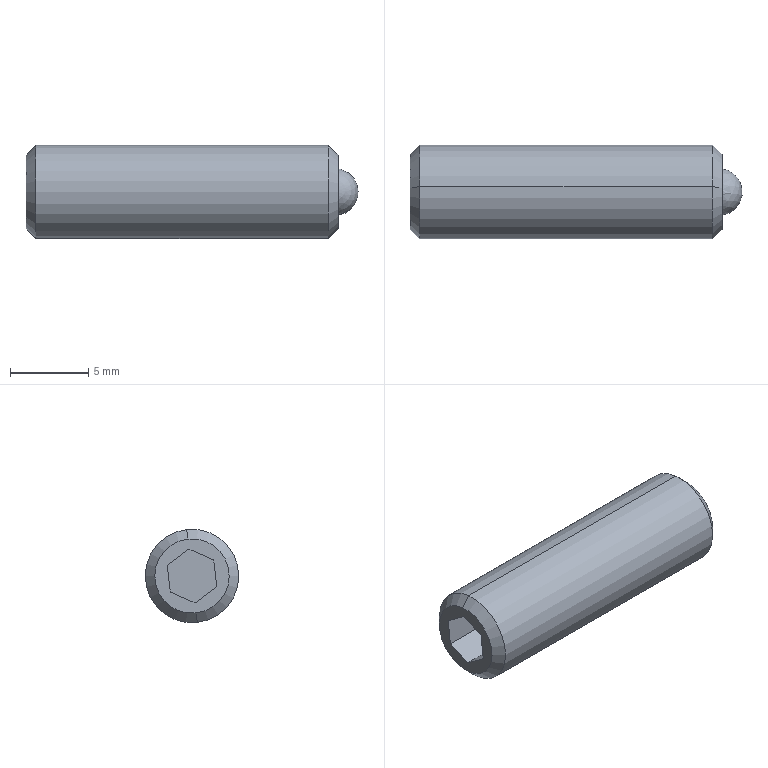Part | NX | features _ZAH01-M6 2 | 1 solid | 16 faces | box 21.3 x 6 x 6 mm | volume 545.053 mm3 | plane 9 | cone 4 | cylinder 2 | sphere 1 | commonest cylinder face diameters 6 x2
STEP:
#1=CARTESIAN_POINT('',(-46.614,117.663,-91.481));
#2=VERTEX_POINT('',#1);
#3=CARTESIAN_POINT('',(-46.614,118.337,-85.519));
#4=VERTEX_POINT('',#3);
#5=CARTESIAN_POINT('',(-46.614,118.,-88.5));
#6=DIRECTION('',(-1.,0.,0.));
#7=DIRECTION('',(0.,-0.1124,-0.9937));
#8=AXIS2_PLACEMENT_3D('',#5,#6,#7);
#9=CIRCLE('',#8,3.);
#10=EDGE_CURVE('',#2,#4,#9,.T.);
#11=ORIENTED_EDGE('',*,*,#10,.T.);
#12=CARTESIAN_POINT('',(-65.386,118.337,-85.519));
#13=VERTEX_POINT('',#12);
#14=CARTESIAN_POINT('',(-46.,118.337,-85.519));
#15=DIRECTION('',(-1.,0.,0.));
#16=VECTOR('',#15,1000.);
#17=LINE('',#14,#16);
#18=EDGE_CURVE('',#4,#13,#17,.T.);
#19=ORIENTED_EDGE('',*,*,#18,.T.);
#20=CARTESIAN_POINT('',(-65.386,117.663,-91.481));
#21=VERTEX_POINT('',#20);
#22=CARTESIAN_POINT('',(-65.386,118.,-88.5));
#23=DIRECTION('',(1.,0.,0.));
#24=DIRECTION('',(0.,-0.1124,-0.9937));
#25=AXIS2_PLACEMENT_3D('',#22,#23,#24);
#26=CIRCLE('',#25,3.);
#27=EDGE_CURVE('',#13,#21,#26,.T.);
#28=ORIENTED_EDGE('',*,*,#27,.T.);
#29=CARTESIAN_POINT('',(-46.,117.663,-91.481));
#30=DIRECTION('',(-1.,0.,0.));
#31=VECTOR('',#30,1000.);
#32=LINE('',#29,#31);
#33=EDGE_CURVE('',#21,#2,#32,.F.);
#34=ORIENTED_EDGE('',*,*,#33,.T.);
#35=EDGE_LOOP('',(#11,#19,#28,#34));
#36=FACE_BOUND('',#35,.T.);
#37=CARTESIAN_POINT('',(-46.,118.,-88.5));
#38=DIRECTION('',(-1.,0.,0.));
#39=DIRECTION('',(0.,0.1124,0.9937));
#40=AXIS2_PLACEMENT_3D('',#37,#38,#39);
#41=CYLINDRICAL_SURFACE('',#40,3.);
#42=ADVANCED_FACE('',(#36),#41,.T.);
#43=CARTESIAN_POINT('',(-66.,118.268,-86.129));
#44=VERTEX_POINT('',#43);
#45=CARTESIAN_POINT('',(-66.,117.732,-90.871));
#46=VERTEX_POINT('',#45);
#47=CARTESIAN_POINT('',(-66.,118.,-88.5));
#48=DIRECTION('',(1.,0.,0.));
#49=DIRECTION('',(0.,0.1124,0.9937));
#50=AXIS2_PLACEMENT_3D('',#47,#48,#49);
#51=CIRCLE('',#50,2.387);
#52=EDGE_CURVE('',#44,#46,#51,.T.);
#53=ORIENTED_EDGE('',*,*,#52,.T.);
#54=CARTESIAN_POINT('',(-65.386,117.663,-91.481));
#55=DIRECTION('',(0.7071,-0.07947,-0.7026));
#56=VECTOR('',#55,1000.);
#57=LINE('',#54,#56);
#58=EDGE_CURVE('',#46,#21,#57,.T.);
#59=ORIENTED_EDGE('',*,*,#58,.T.);
#60=ORIENTED_EDGE('',*,*,#27,.F.);
#61=CARTESIAN_POINT('',(-65.386,118.337,-85.519));
#62=DIRECTION('',(0.7071,0.07947,0.7026));
#63=VECTOR('',#62,1000.);
#64=LINE('',#61,#63);
#65=EDGE_CURVE('',#13,#44,#64,.F.);
#66=ORIENTED_EDGE('',*,*,#65,.T.);
#67=EDGE_LOOP('',(#53,#59,#60,#66));
#68=FACE_BOUND('',#67,.T.);
#69=CARTESIAN_POINT('',(-65.386,118.,-88.5));
#70=DIRECTION('',(1.,0.,0.));
#71=DIRECTION('',(0.,-0.1124,-0.9937));
#72=AXIS2_PLACEMENT_3D('',#69,#70,#71);
#73=CONICAL_SURFACE('',#72,3.,0.7854);
#74=ADVANCED_FACE('',(#68),#73,.T.);
#75=CARTESIAN_POINT('',(-46.,117.732,-90.871));
#76=VERTEX_POINT('',#75);
#77=CARTESIAN_POINT('',(-46.,118.268,-86.129));
#78=VERTEX_POINT('',#77);
#79=CARTESIAN_POINT('',(-46.,118.,-88.5));
#80=DIRECTION('',(-1.,0.,0.));
#81=DIRECTION('',(0.,-0.1124,-0.9937));
#82=AXIS2_PLACEMENT_3D('',#79,#80,#81);
#83=CIRCLE('',#82,2.387);
#84=EDGE_CURVE('',#76,#78,#83,.T.);
#85=ORIENTED_EDGE('',*,*,#84,.T.);
#86=CARTESIAN_POINT('',(-46.614,118.337,-85.519));
#87=DIRECTION('',(-0.7071,0.07947,0.7026));
#88=VECTOR('',#87,1000.);
#89=LINE('',#86,#88);
#90=EDGE_CURVE('',#4,#78,#89,.F.);
#91=ORIENTED_EDGE('',*,*,#90,.F.);
#92=ORIENTED_EDGE('',*,*,#10,.F.);
#93=CARTESIAN_POINT('',(-46.614,117.663,-91.481));
#94=DIRECTION('',(-0.7071,-0.07947,-0.7026));
#95=VECTOR('',#94,1000.);
#96=LINE('',#93,#95);
#97=EDGE_CURVE('',#76,#2,#96,.T.);
#98=ORIENTED_EDGE('',*,*,#97,.F.);
#99=EDGE_LOOP('',(#85,#91,#92,#98));
#100=FACE_BOUND('',#99,.T.);
#101=CARTESIAN_POINT('',(-46.614,118.,-88.5));
#102=DIRECTION('',(-1.,0.,0.));
#103=DIRECTION('',(0.,0.1124,0.9937));
#104=AXIS2_PLACEMENT_3D('',#101,#102,#103);
#105=CONICAL_SURFACE('',#104,3.,0.7854);
#106=ADVANCED_FACE('',(#100),#105,.T.);
#107=ORIENTED_EDGE('',*,*,#18,.F.);
#108=CARTESIAN_POINT('',(-46.614,118.,-88.5));
#109=DIRECTION('',(-1.,0.,0.));
#110=DIRECTION('',(0.,-0.1124,-0.9937));
#111=AXIS2_PLACEMENT_3D('',#108,#109,#110);
#112=CIRCLE('',#111,3.);
#113=EDGE_CURVE('',#4,#2,#112,.T.);
#114=ORIENTED_EDGE('',*,*,#113,.T.);
#115=ORIENTED_EDGE('',*,*,#33,.F.);
#116=CARTESIAN_POINT('',(-65.386,118.,-88.5));
#117=DIRECTION('',(1.,0.,0.));
#118=DIRECTION('',(0.,-0.1124,-0.9937));
#119=AXIS2_PLACEMENT_3D('',#116,#117,#118);
#120=CIRCLE('',#119,3.);
#121=EDGE_CURVE('',#21,#13,#120,.T.);
#122=ORIENTED_EDGE('',*,*,#121,.T.);
#123=EDGE_LOOP('',(#107,#114,#115,#122));
#124=FACE_BOUND('',#123,.T.);
#125=CARTESIAN_POINT('',(-46.,118.,-88.5));
#126=DIRECTION('',(-1.,0.,0.));
#127=DIRECTION('',(0.,0.1124,0.9937));
#128=AXIS2_PLACEMENT_3D('',#125,#126,#127);
#129=CYLINDRICAL_SURFACE('',#128,3.);
#130=ADVANCED_FACE('',(#124),#129,.T.);
#131=ORIENTED_EDGE('',*,*,#58,.F.);
#132=CARTESIAN_POINT('',(-66.,118.,-88.5));
#133=DIRECTION('',(1.,0.,0.));
#134=DIRECTION('',(0.,0.1124,0.9937));
#135=AXIS2_PLACEMENT_3D('',#132,#133,#134);
#136=CIRCLE('',#135,2.387);
#137=EDGE_CURVE('',#46,#44,#136,.T.);
#138=ORIENTED_EDGE('',*,*,#137,.T.);
#139=ORIENTED_EDGE('',*,*,#65,.F.);
#140=ORIENTED_EDGE('',*,*,#121,.F.);
#141=EDGE_LOOP('',(#131,#138,#139,#140));
#142=FACE_BOUND('',#141,.T.);
#143=CARTESIAN_POINT('',(-65.386,118.,-88.5));
#144=DIRECTION('',(1.,0.,0.));
#145=DIRECTION('',(0.,-0.1124,-0.9937));
#146=AXIS2_PLACEMENT_3D('',#143,#144,#145);
#147=CONICAL_SURFACE('',#146,3.,0.7854);
#148=ADVANCED_FACE('',(#142),#147,.T.);
#149=ORIENTED_EDGE('',*,*,#90,.T.);
#150=CARTESIAN_POINT('',(-46.,118.,-88.5));
#151=DIRECTION('',(-1.,0.,0.));
#152=DIRECTION('',(0.,-0.1124,-0.9937));
#153=AXIS2_PLACEMENT_3D('',#150,#151,#152);
#154=CIRCLE('',#153,2.387);
#155=EDGE_CURVE('',#78,#76,#154,.T.);
#156=ORIENTED_EDGE('',*,*,#155,.T.);
#157=ORIENTED_EDGE('',*,*,#97,.T.);
#158=ORIENTED_EDGE('',*,*,#113,.F.);
#159=EDGE_LOOP('',(#149,#156,#157,#158));
#160=FACE_BOUND('',#159,.T.);
#161=CARTESIAN_POINT('',(-46.614,118.,-88.5));
#162=DIRECTION('',(-1.,0.,0.));
#163=DIRECTION('',(0.,0.1124,0.9937));
#164=AXIS2_PLACEMENT_3D('',#161,#162,#163);
#165=CONICAL_SURFACE('',#164,3.,0.7854);
#166=ADVANCED_FACE('',(#160),#165,.T.);
#167=CARTESIAN_POINT('',(-66.,118.195,-86.779));
#168=VERTEX_POINT('',#167);
#169=CARTESIAN_POINT('',(-66.,116.607,-87.471));
#170=VERTEX_POINT('',#169);
#171=CARTESIAN_POINT('',(-66.,116.607,-87.471));
#172=DIRECTION('',(0.,-0.9167,-0.3995));
#173=VECTOR('',#172,1000.);
#174=LINE('',#171,#173);
#175=EDGE_CURVE('',#168,#170,#174,.T.);
#176=ORIENTED_EDGE('',*,*,#175,.T.);
#177=CARTESIAN_POINT('',(-66.,116.412,-89.192));
#178=VERTEX_POINT('',#177);
#179=CARTESIAN_POINT('',(-66.,116.412,-89.192));
#180=DIRECTION('',(0.,-0.1124,-0.9937));
#181=VECTOR('',#180,1000.);
#182=LINE('',#179,#181);
#183=EDGE_CURVE('',#170,#178,#182,.T.);
#184=ORIENTED_EDGE('',*,*,#183,.T.);
#185=CARTESIAN_POINT('',(-66.,117.805,-90.221));
#186=VERTEX_POINT('',#185);
#187=CARTESIAN_POINT('',(-66.,117.805,-90.221));
#188=DIRECTION('',(0.,0.8043,-0.5942));
#189=VECTOR('',#188,1000.);
#190=LINE('',#187,#189);
#191=EDGE_CURVE('',#178,#186,#190,.T.);
#192=ORIENTED_EDGE('',*,*,#191,.T.);
#193=CARTESIAN_POINT('',(-66.,119.393,-89.529));
#194=VERTEX_POINT('',#193);
#195=CARTESIAN_POINT('',(-66.,119.393,-89.529));
#196=DIRECTION('',(0.,0.9167,0.3995));
#197=VECTOR('',#196,1000.);
#198=LINE('',#195,#197);
#199=EDGE_CURVE('',#186,#194,#198,.T.);
#200=ORIENTED_EDGE('',*,*,#199,.T.);
#201=CARTESIAN_POINT('',(-66.,119.588,-87.808));
#202=VERTEX_POINT('',#201);
#203=CARTESIAN_POINT('',(-66.,119.588,-87.808));
#204=DIRECTION('',(0.,0.1124,0.9937));
#205=VECTOR('',#204,1000.);
#206=LINE('',#203,#205);
#207=EDGE_CURVE('',#194,#202,#206,.T.);
#208=ORIENTED_EDGE('',*,*,#207,.T.);
#209=CARTESIAN_POINT('',(-66.,118.195,-86.779));
#210=DIRECTION('',(0.,0.8043,-0.5942));
#211=VECTOR('',#210,1000.);
#212=LINE('',#209,#211);
#213=EDGE_CURVE('',#168,#202,#212,.T.);
#214=ORIENTED_EDGE('',*,*,#213,.F.);
#215=EDGE_LOOP('',(#176,#184,#192,#200,#208,#214));
#216=FACE_BOUND('',#215,.T.);
#217=ORIENTED_EDGE('',*,*,#52,.F.);
#218=ORIENTED_EDGE('',*,*,#137,.F.);
#219=EDGE_LOOP('',(#217,#218));
#220=FACE_BOUND('',#219,.T.);
#221=CARTESIAN_POINT('',(-66.,118.,-88.5));
#222=DIRECTION('',(1.,0.,0.));
#223=DIRECTION('',(0.,-0.1124,-0.9937));
#224=AXIS2_PLACEMENT_3D('',#221,#222,#223);
#225=PLANE('',#224);
#226=ADVANCED_FACE('',(#216,#220),#225,.F.);
#227=ORIENTED_EDGE('',*,*,#84,.F.);
#228=ORIENTED_EDGE('',*,*,#155,.F.);
#229=EDGE_LOOP('',(#227,#228));
#230=FACE_BOUND('',#229,.T.);
#231=CARTESIAN_POINT('',(-46.,118.167,-87.023));
#232=VERTEX_POINT('',#231);
#233=CARTESIAN_POINT('',(-46.,117.832,-89.977));
#234=VERTEX_POINT('',#233);
#235=CARTESIAN_POINT('',(-46.,118.,-88.5));
#236=DIRECTION('',(-1.,0.,0.));
#237=DIRECTION('',(0.,-0.1124,-0.9937));
#238=AXIS2_PLACEMENT_3D('',#235,#236,#237);
#239=CIRCLE('',#238,1.487);
#240=EDGE_CURVE('',#232,#234,#239,.F.);
#241=ORIENTED_EDGE('',*,*,#240,.F.);
#242=CARTESIAN_POINT('',(-46.,118.,-88.5));
#243=DIRECTION('',(-1.,0.,0.));
#244=DIRECTION('',(0.,-0.1124,-0.9937));
#245=AXIS2_PLACEMENT_3D('',#242,#243,#244);
#246=CIRCLE('',#245,1.487);
#247=EDGE_CURVE('',#234,#232,#246,.F.);
#248=ORIENTED_EDGE('',*,*,#247,.F.);
#249=EDGE_LOOP('',(#241,#248));
#250=FACE_BOUND('',#249,.T.);
#251=CARTESIAN_POINT('',(-46.,120.371,-88.768));
#252=DIRECTION('',(-1.,0.,0.));
#253=DIRECTION('',(0.,0.1124,0.9937));
#254=AXIS2_PLACEMENT_3D('',#251,#252,#253);
#255=PLANE('',#254);
#256=ADVANCED_FACE('',(#230,#250),#255,.F.);
#257=CARTESIAN_POINT('',(-63.5,119.588,-87.808));
#258=VERTEX_POINT('',#257);
#259=CARTESIAN_POINT('',(-63.5,119.588,-87.808));
#260=DIRECTION('',(-1.,0.,0.));
#261=VECTOR('',#260,1000.);
#262=LINE('',#259,#261);
#263=EDGE_CURVE('',#258,#202,#262,.T.);
#264=ORIENTED_EDGE('',*,*,#263,.F.);
#265=CARTESIAN_POINT('',(-63.5,118.195,-86.779));
#266=VERTEX_POINT('',#265);
#267=CARTESIAN_POINT('',(-63.5,118.195,-86.779));
#268=DIRECTION('',(0.,0.8043,-0.5942));
#269=VECTOR('',#268,1000.);
#270=LINE('',#267,#269);
#271=EDGE_CURVE('',#266,#258,#270,.T.);
#272=ORIENTED_EDGE('',*,*,#271,.F.);
#273=CARTESIAN_POINT('',(-63.5,118.195,-86.779));
#274=DIRECTION('',(1.,0.,0.));
#275=VECTOR('',#274,1000.);
#276=LINE('',#273,#275);
#277=EDGE_CURVE('',#168,#266,#276,.T.);
#278=ORIENTED_EDGE('',*,*,#277,.F.);
#279=ORIENTED_EDGE('',*,*,#213,.T.);
#280=EDGE_LOOP('',(#264,#272,#278,#279));
#281=FACE_BOUND('',#280,.T.);
#282=CARTESIAN_POINT('',(-63.5,118.195,-86.779));
#283=DIRECTION('',(0.,0.5942,0.8043));
#284=DIRECTION('',(0.,0.8043,-0.5942));
#285=AXIS2_PLACEMENT_3D('',#282,#283,#284);
#286=PLANE('',#285);
#287=ADVANCED_FACE('',(#281),#286,.F.);
#288=ORIENTED_EDGE('',*,*,#240,.T.);
#289=ORIENTED_EDGE('',*,*,#247,.T.);
#290=EDGE_LOOP('',(#288,#289));
#291=FACE_BOUND('',#290,.T.);
#292=CARTESIAN_POINT('',(-46.2,118.,-88.5));
#293=DIRECTION('',(0.,-0.9937,0.1124));
#294=DIRECTION('',(0.1154,-0.1116,-0.987));
#295=AXIS2_PLACEMENT_3D('',#292,#293,#294);
#296=SPHERICAL_SURFACE('',#295,1.5);
#297=ADVANCED_FACE('',(#291),#296,.T.);
#298=ORIENTED_EDGE('',*,*,#207,.F.);
#299=CARTESIAN_POINT('',(-63.5,119.393,-89.529));
#300=VERTEX_POINT('',#299);
#301=CARTESIAN_POINT('',(-63.5,119.393,-89.529));
#302=DIRECTION('',(-1.,0.,0.));
#303=VECTOR('',#302,1000.);
#304=LINE('',#301,#303);
#305=EDGE_CURVE('',#300,#194,#304,.T.);
#306=ORIENTED_EDGE('',*,*,#305,.F.);
#307=CARTESIAN_POINT('',(-63.5,119.588,-87.808));
#308=DIRECTION('',(0.,-0.1124,-0.9937));
#309=VECTOR('',#308,1000.);
#310=LINE('',#307,#309);
#311=EDGE_CURVE('',#258,#300,#310,.T.);
#312=ORIENTED_EDGE('',*,*,#311,.F.);
#313=ORIENTED_EDGE('',*,*,#263,.T.);
#314=EDGE_LOOP('',(#298,#306,#312,#313));
#315=FACE_BOUND('',#314,.T.);
#316=CARTESIAN_POINT('',(-63.5,119.588,-87.808));
#317=DIRECTION('',(0.,0.9937,-0.1124));
#318=DIRECTION('',(1.,0.,0.));
#319=AXIS2_PLACEMENT_3D('',#316,#317,#318);
#320=PLANE('',#319);
#321=ADVANCED_FACE('',(#315),#320,.F.);
#322=CARTESIAN_POINT('',(-63.5,117.805,-90.221));
#323=VERTEX_POINT('',#322);
#324=CARTESIAN_POINT('',(-63.5,119.393,-89.529));
#325=DIRECTION('',(0.,-0.9167,-0.3995));
#326=VECTOR('',#325,1000.);
#327=LINE('',#324,#326);
#328=EDGE_CURVE('',#300,#323,#327,.T.);
#329=ORIENTED_EDGE('',*,*,#328,.T.);
#330=CARTESIAN_POINT('',(-63.5,116.412,-89.192));
#331=VERTEX_POINT('',#330);
#332=CARTESIAN_POINT('',(-63.5,117.805,-90.221));
#333=DIRECTION('',(0.,-0.8043,0.5942));
#334=VECTOR('',#333,1000.);
#335=LINE('',#332,#334);
#336=EDGE_CURVE('',#323,#331,#335,.T.);
#337=ORIENTED_EDGE('',*,*,#336,.T.);
#338=CARTESIAN_POINT('',(-63.5,116.607,-87.471));
#339=VERTEX_POINT('',#338);
#340=CARTESIAN_POINT('',(-63.5,116.412,-89.192));
#341=DIRECTION('',(0.,0.1124,0.9937));
#342=VECTOR('',#341,1000.);
#343=LINE('',#340,#342);
#344=EDGE_CURVE('',#331,#339,#343,.T.);
#345=ORIENTED_EDGE('',*,*,#344,.T.);
#346=CARTESIAN_POINT('',(-63.5,116.607,-87.471));
#347=DIRECTION('',(0.,0.9167,0.3995));
#348=VECTOR('',#347,1000.);
#349=LINE('',#346,#348);
#350=EDGE_CURVE('',#339,#266,#349,.T.);
#351=ORIENTED_EDGE('',*,*,#350,.T.);
#352=ORIENTED_EDGE('',*,*,#271,.T.);
#353=ORIENTED_EDGE('',*,*,#311,.T.);
#354=EDGE_LOOP('',(#329,#337,#345,#351,#352,#353));
#355=FACE_BOUND('',#354,.T.);
#356=CARTESIAN_POINT('',(-63.5,118.,-88.5));
#357=DIRECTION('',(-1.,0.,0.));
#358=DIRECTION('',(0.,0.1124,0.9937));
#359=AXIS2_PLACEMENT_3D('',#356,#357,#358);
#360=PLANE('',#359);
#361=ADVANCED_FACE('',(#355),#360,.T.);
#362=ORIENTED_EDGE('',*,*,#277,.T.);
#363=ORIENTED_EDGE('',*,*,#350,.F.);
#364=CARTESIAN_POINT('',(-63.5,116.607,-87.471));
#365=DIRECTION('',(1.,0.,0.));
#366=VECTOR('',#365,1000.);
#367=LINE('',#364,#366);
#368=EDGE_CURVE('',#170,#339,#367,.T.);
#369=ORIENTED_EDGE('',*,*,#368,.F.);
#370=ORIENTED_EDGE('',*,*,#175,.F.);
#371=EDGE_LOOP('',(#362,#363,#369,#370));
#372=FACE_BOUND('',#371,.T.);
#373=CARTESIAN_POINT('',(-63.5,116.607,-87.471));
#374=DIRECTION('',(0.,-0.3995,0.9167));
#375=DIRECTION('',(0.,0.9167,0.3995));
#376=AXIS2_PLACEMENT_3D('',#373,#374,#375);
#377=PLANE('',#376);
#378=ADVANCED_FACE('',(#372),#377,.F.);
#379=CARTESIAN_POINT('',(-63.5,117.805,-90.221));
#380=DIRECTION('',(-1.,0.,0.));
#381=VECTOR('',#380,1000.);
#382=LINE('',#379,#381);
#383=EDGE_CURVE('',#323,#186,#382,.T.);
#384=ORIENTED_EDGE('',*,*,#383,.F.);
#385=ORIENTED_EDGE('',*,*,#328,.F.);
#386=ORIENTED_EDGE('',*,*,#305,.T.);
#387=ORIENTED_EDGE('',*,*,#199,.F.);
#388=EDGE_LOOP('',(#384,#385,#386,#387));
#389=FACE_BOUND('',#388,.T.);
#390=CARTESIAN_POINT('',(-63.5,119.393,-89.529));
#391=DIRECTION('',(0.,0.3995,-0.9167));
#392=DIRECTION('',(0.,-0.9167,-0.3995));
#393=AXIS2_PLACEMENT_3D('',#390,#391,#392);
#394=PLANE('',#393);
#395=ADVANCED_FACE('',(#389),#394,.F.);
#396=ORIENTED_EDGE('',*,*,#368,.T.);
#397=ORIENTED_EDGE('',*,*,#344,.F.);
#398=CARTESIAN_POINT('',(-63.5,116.412,-89.192));
#399=DIRECTION('',(1.,0.,0.));
#400=VECTOR('',#399,1000.);
#401=LINE('',#398,#400);
#402=EDGE_CURVE('',#178,#331,#401,.T.);
#403=ORIENTED_EDGE('',*,*,#402,.F.);
#404=ORIENTED_EDGE('',*,*,#183,.F.);
#405=EDGE_LOOP('',(#396,#397,#403,#404));
#406=FACE_BOUND('',#405,.T.);
#407=CARTESIAN_POINT('',(-63.5,116.412,-89.192));
#408=DIRECTION('',(0.,-0.9937,0.1124));
#409=DIRECTION('',(-1.,0.,0.));
#410=AXIS2_PLACEMENT_3D('',#407,#408,#409);
#411=PLANE('',#410);
#412=ADVANCED_FACE('',(#406),#411,.F.);
#413=ORIENTED_EDGE('',*,*,#402,.T.);
#414=ORIENTED_EDGE('',*,*,#336,.F.);
#415=ORIENTED_EDGE('',*,*,#383,.T.);
#416=ORIENTED_EDGE('',*,*,#191,.F.);
#417=EDGE_LOOP('',(#413,#414,#415,#416));
#418=FACE_BOUND('',#417,.T.);
#419=CARTESIAN_POINT('',(-63.5,117.805,-90.221));
#420=DIRECTION('',(0.,-0.5942,-0.8043));
#421=DIRECTION('',(0.,-0.8043,0.5942));
#422=AXIS2_PLACEMENT_3D('',#419,#420,#421);
#423=PLANE('',#422);
#424=ADVANCED_FACE('',(#418),#423,.F.);
#425=CLOSED_SHELL('',(#42,#74,#106,#130,#148,#166,#226,#256,#287,#297,#321,#361,#378,#395,#412,#424));
#426=MANIFOLD_SOLID_BREP('',#425);
#427=(LENGTH_UNIT()NAMED_UNIT(*)SI_UNIT(.MILLI.,.METRE.));
#428=UNCERTAINTY_MEASURE_WITH_UNIT(LENGTH_MEASURE(0.00001),#427,'','');
#429=(NAMED_UNIT(*)PLANE_ANGLE_UNIT()SI_UNIT($,.RADIAN.));
#430=(NAMED_UNIT(*)SI_UNIT($,.STERADIAN.)SOLID_ANGLE_UNIT());
#431=(GEOMETRIC_REPRESENTATION_CONTEXT(3)GLOBAL_UNCERTAINTY_ASSIGNED_CONTEXT((#428))GLOBAL_UNIT_ASSIGNED_CONTEXT((#427,#429,#430))REPRESENTATION_CONTEXT('',''));
#432=ADVANCED_BREP_SHAPE_REPRESENTATION('',(#426),#431);